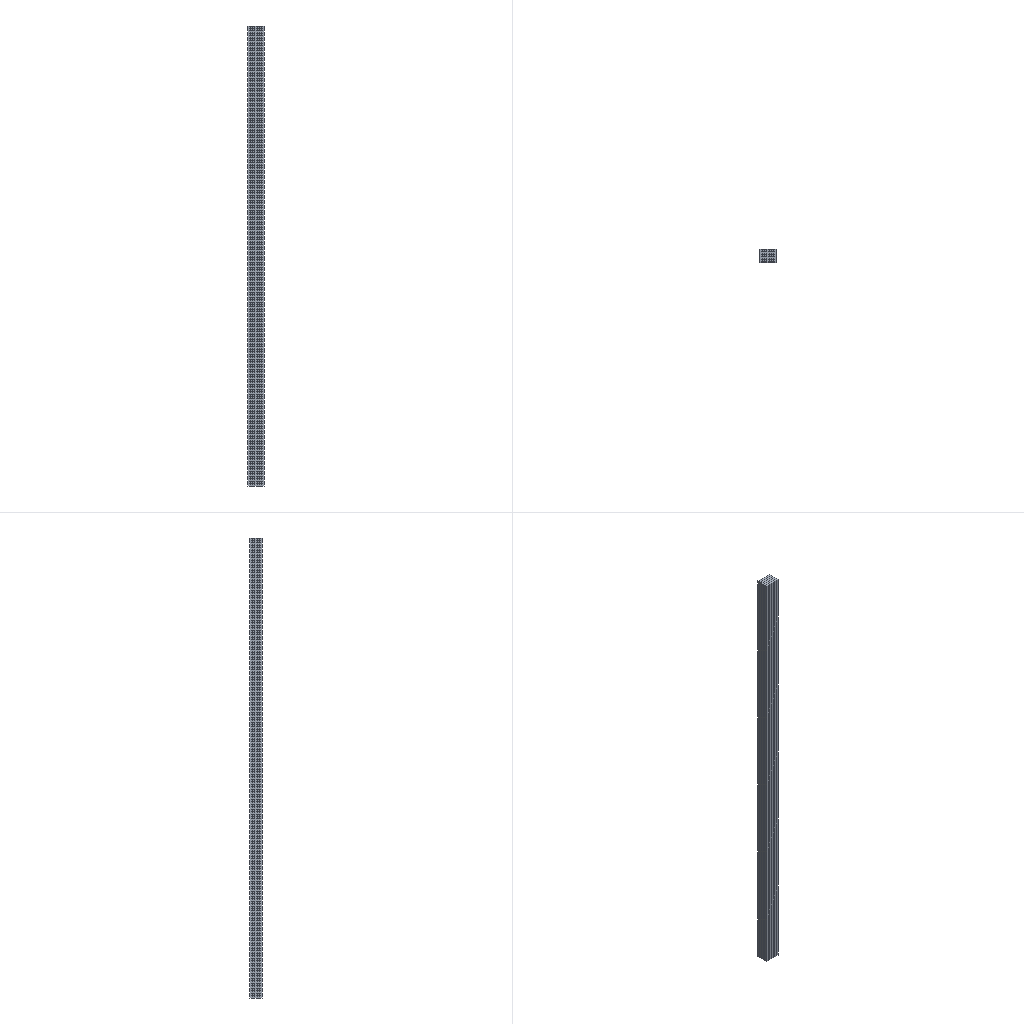Simulation study | abaqus
Set-up summary:
category,name,step,type,value,unit,region
solver,abaqus
solver,version,,,Abaqus/Standard 3DEXPERIENCE R2017x
units,not stated in the deck,,not stated
analysis,deck,,coupled temperature-displacement,coupled temperature-displacement
load_step,Step-1,Step-1,coupled temperature-displacement
load_step,requested,,,1
mesh,nodes,,,8928
mesh,elements,,,6475
element_type,C3D8T,,solid,6475
load,load commands in deck,,count,4
bc,support commands in deck,,count,1
material,MATERIAL-1,,in results
check,setup vs results,,match,"per instance, exact: element labels, types and connectivity; labels of the nodes the elements use; coordinates of those nodes at SINGLE_PRECISION in 1 of 1 instance(s)"
Abaqus input file, long lists of numbers shortened:
*Heading
** Job name: Job-1 Model name: Job-1
** Generated by: Abaqus/CAE 2017
*Preprint, echo=NO, model=NO, history=NO, contact=NO
**
** PARTS
**
*Part, name=PART-1
*Node
      1,           0.,        -100.,        3700.
      2,           0.,         -80.,        3700.
** (8926 more lines like these left out)
*Element, type=C3D8T
   1, 1117, 1118, 1124, 1123,    1,    2,    8,    7
   2, 1118, 1119, 1125, 1124,    2,    3,    9,    8
** (6473 more lines like these left out)
*Nset, nset=SET-1, generate
    1,  8928,     1
*Elset, elset=SET-1, generate
    1,  6475,     1
*Orientation, name=Ori-1
          1.,           0.,           0.,           0.,           1.,           0.
1, 0.
** Section: Section-1-SET-1
*Solid Section, elset=SET-1, orientation=Ori-1, material=MATERIAL-1
,
*End Part
**
**
** ASSEMBLY
**
*Assembly, name=Assembly
**
*Instance, name=PART-1-1, part=PART-1
*End Instance
**
*Nset, nset=SET-1, instance=PART-1-1, generate
    1,  8928,     1
*Elset, elset=SET-1, instance=PART-1-1, generate
    1,  6475,     1
*Nset, nset=SET-2, instance=PART-1-1
    1,    2,    3,    4,    5,    6, 1111, 1112, 1113, 1114, 1115, 1116, 1117, 1118, 1119, 1120
 1121, 1122, 2227, 2228, 2229, 2230, 2231, 2232, 2233, 2234, 2235, 2236, 2237, 2238, 3343, 3344
** (4 more lines like these left out)
*Elset, elset=SET-2, instance=PART-1-1
    1,    2,    3,    4,    5,  921,  922,  923,  924,  925,  926,  927,  928,  929,  930, 1846
 1847, 1848, 1849, 1850, 1851, 1852, 1853, 1854, 1855, 2771, 2772, 2773, 2774, 2775, 2776, 2777
** (3 more lines like these left out)
*Nset, nset=SET-3, instance=PART-1-1, generate
    1,  8928,     1
*Elset, elset=SET-3, instance=PART-1-1, generate
    1,  6475,     1
*Nset, nset=SET-4, instance=PART-1-1, generate
    1,  8928,     1
*Elset, elset=SET-4, instance=PART-1-1, generate
    1,  6475,     1
*Nset, nset=SET-5, instance=PART-1-1, generate
    1,  8928,     1
*Elset, elset=SET-5, instance=PART-1-1, generate
    1,  6475,     1
*Nset, nset=SET-6, instance=PART-1-1, generate
    1,  8928,     1
*Elset, elset=SET-6, instance=PART-1-1, generate
    1,  6475,     1
*Nset, nset=SET-7, instance=PART-1-1, generate
    1,  8928,     1
*Elset, elset=SET-7, instance=PART-1-1, generate
    1,  6475,     1
*Elset, elset=_SURF-1_S1, internal, instance=PART-1-1, generate
 5551,  6475,     1
*Elset, elset=_SURF-1_S2, internal, instance=PART-1-1, generate
   1,  925,    1
*Elset, elset=_SURF-1_S4, internal, instance=PART-1-1, generate
    5,  6475,     5
*Elset, elset=_SURF-2_S1, internal, instance=PART-1-1, generate
 5551,  6475,     1
*Elset, elset=_SURF-2_S2, internal, instance=PART-1-1, generate
   1,  925,    1
*Elset, elset=_SURF-2_S4, internal, instance=PART-1-1, generate
    5,  6475,     5
*Elset, elset=_SURF-3_S6, internal, instance=PART-1-1, generate
    1,  6471,     5
*Elset, elset=_SURF-4_S1, internal, instance=PART-1-1, generate
 5551,  6475,     1
*Elset, elset=_SURF-4_S2, internal, instance=PART-1-1, generate
   1,  925,    1
*Elset, elset=_SURF-4_S3, internal, instance=PART-1-1
    1,    2,    3,    4,    5,  926,  927,  928,  929,  930, 1851, 1852, 1853, 1854, 1855, 2776
 2777, 2778, 2779, 2780, 3701, 3702, 3703, 3704, 3705, 4626, 4627, 4628, 4629, 4630, 5551, 5552
** (1 more lines like these left out)
*Elset, elset=_SURF-4_S4, internal, instance=PART-1-1, generate
    5,  6475,     5
*Elset, elset=_SURF-4_S5, internal, instance=PART-1-1
  921,  922,  923,  924,  925, 1846, 1847, 1848, 1849, 1850, 2771, 2772, 2773, 2774, 2775, 3696
 3697, 3698, 3699, 3700, 4621, 4622, 4623, 4624, 4625, 5546, 5547, 5548, 5549, 5550, 6471, 6472
** (1 more lines like these left out)
*Elset, elset=_SURF-4_S6, internal, instance=PART-1-1, generate
    1,  6471,     5
*Elset, elset=_SURF-5_S1, internal, instance=PART-1-1, generate
 5551,  6475,     1
*Elset, elset=_SURF-5_S2, internal, instance=PART-1-1, generate
   1,  925,    1
*Elset, elset=_SURF-5_S6, internal, instance=PART-1-1, generate
    1,  6471,     5
*Elset, elset=_SURF-1_S1_1, internal, instance=PART-1-1, generate
 5551,  6475,     1
*Elset, elset=_SURF-1_S2_1, internal, instance=PART-1-1, generate
   1,  925,    1
*Elset, elset=_SURF-1_S4_1, internal, instance=PART-1-1, generate
    5,  6475,     5
*Surface, type=ELEMENT, name=SURF-1
_SURF-1_S1_1, S1
_SURF-1_S2_1, S2
_SURF-1_S4_1, S4
*Elset, elset=_SURF-2_S1_1, internal, instance=PART-1-1, generate
 5551,  6475,     1
*Elset, elset=_SURF-2_S2_1, internal, instance=PART-1-1, generate
   1,  925,    1
*Elset, elset=_SURF-2_S4_1, internal, instance=PART-1-1, generate
    5,  6475,     5
*Surface, type=ELEMENT, name=SURF-2
_SURF-2_S1_1, S1
_SURF-2_S2_1, S2
_SURF-2_S4_1, S4
*Surface, type=ELEMENT, name=SURF-3
_SURF-3_S6, S6
*Elset, elset=_SURF-4_S1_1, internal, instance=PART-1-1, generate
 5551,  6475,     1
*Elset, elset=_SURF-4_S6_1, internal, instance=PART-1-1, generate
    1,  6471,     5
*Elset, elset=_SURF-4_S2_1, internal, instance=PART-1-1, generate
   1,  925,    1
*Elset, elset=_SURF-4_S4_1, internal, instance=PART-1-1, generate
    5,  6475,     5
*Elset, elset=_SURF-4_S3_1, internal, instance=PART-1-1
    1,    2,    3,    4,    5,  926,  927,  928,  929,  930, 1851, 1852, 1853, 1854, 1855, 2776
 2777, 2778, 2779, 2780, 3701, 3702, 3703, 3704, 3705, 4626, 4627, 4628, 4629, 4630, 5551, 5552
** (1 more lines like these left out)
*Elset, elset=_SURF-4_S5_1, internal, instance=PART-1-1
  921,  922,  923,  924,  925, 1846, 1847, 1848, 1849, 1850, 2771, 2772, 2773, 2774, 2775, 3696
 3697, 3698, 3699, 3700, 4621, 4622, 4623, 4624, 4625, 5546, 5547, 5548, 5549, 5550, 6471, 6472
** (1 more lines like these left out)
*Surface, type=ELEMENT, name=SURF-4
_SURF-4_S1_1, S1
_SURF-4_S6_1, S6
_SURF-4_S2_1, S2
_SURF-4_S4_1, S4
_SURF-4_S3_1, S3
_SURF-4_S5_1, S5
*Elset, elset=_SURF-5_S1_1, internal, instance=PART-1-1, generate
 5551,  6475,     1
*Elset, elset=_SURF-5_S6_1, internal, instance=PART-1-1, generate
    1,  6471,     5
*Elset, elset=_SURF-5_S2_1, internal, instance=PART-1-1, generate
   1,  925,    1
*Surface, type=ELEMENT, name=SURF-5
_SURF-5_S1_1, S1
_SURF-5_S6_1, S6
_SURF-5_S2_1, S2
*End Assembly
*Amplitude, name=AMP-1
             0.,             20.,              1.,     349.214,              2.,     444.505,              3.,      502.289
             4.,     543.887,              5.,     576.41,              6.,     603.118,              7.,     625.777
             8.,      645.455,              9.,     662.846,             10.,     678.427,             11.,     692.54
            12.,     705.436,             13.,     717.31,             14.,      728.312,             15.,     738.561
            16.,     748.153,             17.,     757.169,             18.,     765.672,             19.,     773.719
            20.,     781.355,             21.,     788.621,             22.,     795.551,             23.,     802.174
            24.,     808.517,             25.,     814.603,             26.,     820.45,             27.,     826.079
            28.,     831.503,             29.,     836.738,             30.,     841.796,             31.,     846.689
            32.,     851.427,             33.,     856.02,             34.,     860.476,             35.,     864.804
            36.,     869.01,             37.,      873.101,             38.,     877.083,             39.,     880.963
            40.,     884.744,             41.,     888.433,             42.,     892.032,             43.,     895.548
            44.,     898.982,             45.,     902.34,             46.,     905.624,             47.,     908.838
            48.,     911.984,             49.,     915.065,             50.,     918.085,             51.,     921.045
            52.,      923.947,             53.,     926.794,             54.,     929.588,             55.,     932.331
            56.,     935.025,             57.,      937.671,             58.,     940.271,             59.,     942.827
            60.,     945.34,             61.,     947.812,             62.,     950.243,             63.,     952.636
            64.,      954.99,             65.,     957.309,             66.,     959.592,             67.,     961.841
            68.,     964.057,             69.,     966.24,             70.,     968.392,             71.,     970.514
            72.,     972.606,             73.,     974.669,             74.,     976.704,             75.,     978.712
            76.,      980.693,             77.,     982.648,             78.,      984.579,             79.,       986.484
            80.,     988.366,             81.,     990.224,             82.,     992.06,             83.,     993.873
            84.,     995.665,             85.,     997.436,             86.,     999.186,             87.,     1000.915
            88.,     1002.625,             89.,     1004.316,             90.,     1005.988,             91.,     1007.641
            92.,     1009.276,             93.,     1010.894,             94.,     1012.494,             95.,     1014.078
            96.,     1015.645,             97.,     1017.195,             98.,     1018.73,             99.,      1020.249
           100.,     1021.753
*Amplitude, name=AMP-2
             0.,     0.04396,              1.,     0.1758,              2.,     0.3957,              3.,     0.7034
             4.,      1.099,              5.,     1.583,              6.,     2.154,              7.,     2.814
             8.,     3.561,              9.,     4.396,             10.,      5.319,             11.,     6.331
            12.,     7.43,             13.,     8.617,             14.,     9.892,             15.,     11.254
            16.,     12.705,             17.,     14.244,             18.,     15.87,             19.,     17.585
            20.,     19.387,             21.,     21.278,             22.,     23.256,             23.,     25.322
            24.,     27.477,             25.,     29.719,             26.,     32.049,             27.,     34.467
            28.,     36.972,             29.,     39.566,             30.,     42.248,             31.,     45.018
            32.,     47.875,             33.,      50.821,             34.,     53.854,             35.,     56.975
            36.,     60.185,             37.,     63.482,             38.,     66.867,             39.,     70.34
            40.,     73.901,             41.,      77.55,             42.,     81.287,             43.,     85.111
            44.,     89.024,             45.,      93.025,             46.,     97.113,             47.,     101.29
            48.,     105.554,             49.,      109.906,             50.,     114.346,             51.,     118.875
            52.,     123.491,             53.,     128.195,             54.,     132.987,             55.,     137.866
            56.,      142.834,             57.,     147.89,             58.,     153.033,             59.,     158.265
            60.,     163.584,             61.,     168.992,             62.,     174.487,             63.,     180.07
            64.,     185.742,             65.,     191.501,             66.,     197.348,             67.,     203.283
            68.,      209.305,             69.,     215.416,             70.,     221.615,             71.,     227.902
            72.,     234.276,             73.,     240.739,             74.,     247.289,             75.,     253.927
            76.,     260.654,             77.,     267.468,             78.,     274.37,             79.,     281.36
            80.,     288.438,             81.,     295.604,             82.,     302.858,             83.,      310.199
            84.,     317.629,             85.,     325.147,             86.,     332.752,             87.,     340.446
            88.,     348.227,             89.,     356.096,             90.,     364.053,             91.,     372.099
            92.,     380.232,             93.,     388.453,             94.,     396.762,             95.,     405.158
            96.,     413.643,             97.,     422.216,             98.,      430.876,             99.,     439.625
           100.,     448.461,            101.,     457.386,            102.,     466.398,            103.,     475.498
           104.,     484.687,            105.,     493.963,            106.,     503.327,            107.,     512.779
           108.,     522.318,            109.,      531.946,            110.,      541.662,            111.,     551.466
           112.,     561.357,            113.,     571.337,            114.,     581.404,            115.,     591.559
           116.,     601.803,            117.,     612.134,            118.,     622.553,            119.,     633.06
           120.,     643.655,            121.,     654.338,            122.,     665.109,            123.,     675.967
           124.,     686.914,            125.,     697.949,            126.,     709.071,            127.,     720.282
           128.,     731.58,            129.,     742.966,            130.,     754.44,            131.,     766.003
           132.,     777.653,            133.,     789.391,            134.,     801.217,            135.,     813.13
           136.,     825.132,            137.,     837.222,            138.,     849.399,            139.,     861.665
           140.,      874.018,            141.,     886.46,            142.,     898.989,            143.,     911.606
           144.,     924.312,            145.,     937.105,            146.,     949.986,            147.,     962.955
           148.,     976.011,            149.,     989.156,            150.,     1002.389,            151.,     1015.71
           152.,     1029.118,            153.,     1042.615,            154.,     1056.199,            155.,     1069.871
           156.,     1083.632,            157.,       1097.48,            158.,     1111.416,            159.,     1125.44
** (3186 more lines like these left out)
**
** MATERIALS
**
*Material, name=MATERIAL-1
*Conductivity
 0.16,  20.
  0.2, 200.
 0.15, 400.
 0.28, 600.
  0.4, 800.
 0.87,1000.
  1.5,1200.
*Density
 5e-10,
*Elastic, type=ENGINEERING CONSTANTS
10178.,  692.,  509., 0.292, 0.449,  0.39,  651.,   71.
  794.,
*Expansion
 4e-06,
*Specific Heat
 1.89e+09,  20.
  1.9e+09,  90.
 1.38e+10, 100.
 1.32e+10, 110.
    2e+09, 130.
  1.9e+09, 200.
    7e+08, 300.
  1.2e+09, 400.
  1.7e+09, 600.
  1.9e+09, 800.
    2e+09,1200.
**
** PHYSICAL CONSTANTS
**
*Physical Constants, absolute zero=-273., stefan boltzmann=5.6704e-08
**
** BOUNDARY CONDITIONS
**
** Name: Disp-BC-1 Type: 对称/反对称/完全固定
*Boundary
SET-2, ENCASTRE
**
** PREDEFINED FIELDS
**
** Name: Field-1   Type: Temperature
*Initial Conditions, type=TEMPERATURE
SET-7, 20.
** ----------------------------------------------------------------
**
** STEP: Step-1
**
*Step, name=Step-1, nlgeom=YES, inc=1000000
*Coupled Temperature-displacement, creep=none, deltmx=6000., stabilize=0.0002, allsdtol=0.05, continue=NO
129., 6600., 0.066, 6600.
**
** LOADS
**
** Name: SURFFLUX-1   Type: Surface heat flux
*Dsflux, amplitude=AMP-2
SURF-5, S, 2.4
**
** INTERACTIONS
**
** Interaction: SURFFILM-1
*Sfilm
SURF-2, F, 20., 25.
** Interaction: SURFFILM-2
*Sfilm
SURF-3, F, 20., 9.
** Interaction: SURFRADIATE-1
*Sradiate
SURF-4, R, 20., 0.8
**
** OUTPUT REQUESTS
**
*Restart, write, number interval=1, time marks=NO
**
** FIELD OUTPUT: F-Output-2
**
*Output, field
*Element Output, directions=YES
E, HFL, LE, MISES, PE, PEEQ, S, TEMP, VE
**
** FIELD OUTPUT: F-Output-1
**
*Node Output
NT, U, V
**
** HISTORY OUTPUT: H-Output-1
**
*Output, history, variable=PRESELECT
*End Step
Results summary:
result,step,,completed,increments=175 time=6600.0/6600.0
result,analysis,,,"coupled temperature-displacement, steady state"
result,last_loadstep,,,1
result,primary field,,,"U, NT11"